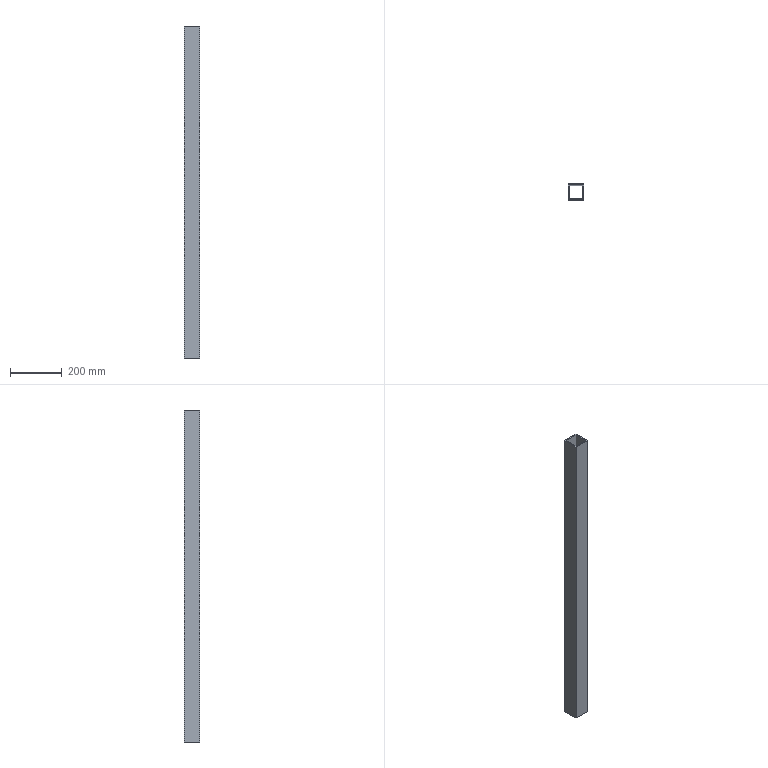Part | STEP file | ASND-0110-E63-HLTP01气SpringLower机架.3 | 1 solid | 10 faces | box 60 x 60 x 1280 mm | volume 1146880 mm3 | plane 10
STEP:
#1=CARTESIAN_POINT('',(0.,0.,0.));
#2=DIRECTION('',(0.,0.,1.));
#3=DIRECTION('',(1.,0.,0.));
#4=AXIS2_PLACEMENT_3D('',#1,#2,#3);
#5=CARTESIAN_POINT('',(-710.,-525.,1280.));
#6=VERTEX_POINT('',#5);
#7=CARTESIAN_POINT('',(-710.,-465.,1280.));
#8=VERTEX_POINT('',#7);
#9=CARTESIAN_POINT('',(-710.,-525.,1280.));
#10=DIRECTION('',(0.,1.,0.));
#11=VECTOR('',#10,1.);
#12=LINE('',#9,#11);
#13=CARTESIAN_POINT('',(-710.,-525.,1364.853));
#14=DIRECTION('',(-1.,0.,0.));
#15=DIRECTION('',(0.,0.7071,0.7071));
#16=AXIS2_PLACEMENT_3D('',#13,#14,#15);
#17=PLANE('',#16);
#18=CARTESIAN_POINT('',(-60.,60.));
#19=DIRECTION('',(0.7071,0.7071));
#20=VECTOR('',#19,1.);
#21=LINE('',#18,#20);
#22=(GEOMETRIC_REPRESENTATION_CONTEXT(2)PARAMETRIC_REPRESENTATION_CONTEXT()REPRESENTATION_CONTEXT('',''));
#23=DEFINITIONAL_REPRESENTATION('',(#21),#22);
#24=PCURVE('',#17,#23);
#25=CARTESIAN_POINT('',(-1564.853,-465.,1280.));
#26=DIRECTION('',(0.,0.,1.));
#27=DIRECTION('',(0.7071,0.7071,0.));
#28=AXIS2_PLACEMENT_3D('',#25,#26,#27);
#29=PLANE('',#28);
#30=CARTESIAN_POINT('',(562.046,-646.899));
#31=DIRECTION('',(0.7071,0.7071));
#32=VECTOR('',#31,1.);
#33=LINE('',#30,#32);
#34=(GEOMETRIC_REPRESENTATION_CONTEXT(2)PARAMETRIC_REPRESENTATION_CONTEXT()REPRESENTATION_CONTEXT('',''));
#35=DEFINITIONAL_REPRESENTATION('',(#33),#34);
#36=PCURVE('',#29,#35);
#37=SURFACE_CURVE('',#12,(#24,#36),.PCURVE_S1.);
#38=EDGE_CURVE('',#6,#8,#37,.T.);
#39=ORIENTED_EDGE('',*,*,#38,.F.);
#40=CARTESIAN_POINT('',(-710.,-525.,0.));
#41=VERTEX_POINT('',#40);
#42=CARTESIAN_POINT('',(-710.,-525.,1280.));
#43=DIRECTION('',(0.,0.,-1.));
#44=VECTOR('',#43,1.);
#45=LINE('',#42,#44);
#46=CARTESIAN_POINT('',(-60.,60.));
#47=DIRECTION('',(-0.7071,0.7071));
#48=VECTOR('',#47,1.);
#49=LINE('',#46,#48);
#50=(GEOMETRIC_REPRESENTATION_CONTEXT(2)PARAMETRIC_REPRESENTATION_CONTEXT()REPRESENTATION_CONTEXT('',''));
#51=DEFINITIONAL_REPRESENTATION('',(#49),#50);
#52=PCURVE('',#17,#51);
#53=CARTESIAN_POINT('',(-770.,-525.,1364.853));
#54=DIRECTION('',(0.,1.,0.));
#55=DIRECTION('',(0.7071,0.,0.7071));
#56=AXIS2_PLACEMENT_3D('',#53,#54,#55);
#57=PLANE('',#56);
#58=CARTESIAN_POINT('',(-17.574,102.426));
#59=DIRECTION('',(-0.7071,0.7071));
#60=VECTOR('',#59,1.);
#61=LINE('',#58,#60);
#62=(GEOMETRIC_REPRESENTATION_CONTEXT(2)PARAMETRIC_REPRESENTATION_CONTEXT()REPRESENTATION_CONTEXT('',''));
#63=DEFINITIONAL_REPRESENTATION('',(#61),#62);
#64=PCURVE('',#57,#63);
#65=SURFACE_CURVE('',#45,(#52,#64),.PCURVE_S1.);
#66=EDGE_CURVE('',#6,#41,#65,.T.);
#67=ORIENTED_EDGE('',*,*,#66,.T.);
#68=CARTESIAN_POINT('',(-710.,-465.,0.));
#69=VERTEX_POINT('',#68);
#70=CARTESIAN_POINT('',(-710.,-525.,0.));
#71=DIRECTION('',(0.,1.,0.));
#72=VECTOR('',#71,1.);
#73=LINE('',#70,#72);
#74=CARTESIAN_POINT('',(-965.097,965.097));
#75=DIRECTION('',(0.7071,0.7071));
#76=VECTOR('',#75,1.);
#77=LINE('',#74,#76);
#78=(GEOMETRIC_REPRESENTATION_CONTEXT(2)PARAMETRIC_REPRESENTATION_CONTEXT()REPRESENTATION_CONTEXT('',''));
#79=DEFINITIONAL_REPRESENTATION('',(#77),#78);
#80=PCURVE('',#17,#79);
#81=CARTESIAN_POINT('',(0.,0.,0.));
#82=DIRECTION('',(0.,0.,1.));
#83=DIRECTION('',(0.7071,0.7071,0.));
#84=AXIS2_PLACEMENT_3D('',#81,#82,#83);
#85=PLANE('',#84);
#86=CARTESIAN_POINT('',(-873.277,130.815));
#87=DIRECTION('',(0.7071,0.7071));
#88=VECTOR('',#87,1.);
#89=LINE('',#86,#88);
#90=(GEOMETRIC_REPRESENTATION_CONTEXT(2)PARAMETRIC_REPRESENTATION_CONTEXT()REPRESENTATION_CONTEXT('',''));
#91=DEFINITIONAL_REPRESENTATION('',(#89),#90);
#92=PCURVE('',#85,#91);
#93=SURFACE_CURVE('',#73,(#80,#92),.PCURVE_S1.);
#94=EDGE_CURVE('',#41,#69,#93,.T.);
#95=ORIENTED_EDGE('',*,*,#94,.T.);
#96=CARTESIAN_POINT('',(-710.,-465.,1280.));
#97=DIRECTION('',(0.,0.,-1.));
#98=VECTOR('',#97,1.);
#99=LINE('',#96,#98);
#100=CARTESIAN_POINT('',(-17.574,102.426));
#101=DIRECTION('',(-0.7071,0.7071));
#102=VECTOR('',#101,1.);
#103=LINE('',#100,#102);
#104=(GEOMETRIC_REPRESENTATION_CONTEXT(2)PARAMETRIC_REPRESENTATION_CONTEXT()REPRESENTATION_CONTEXT('',''));
#105=DEFINITIONAL_REPRESENTATION('',(#103),#104);
#106=PCURVE('',#17,#105);
#107=CARTESIAN_POINT('',(-710.,-465.,1364.853));
#108=DIRECTION('',(0.,-1.,0.));
#109=DIRECTION('',(0.7071,0.,0.7071));
#110=AXIS2_PLACEMENT_3D('',#107,#108,#109);
#111=PLANE('',#110);
#112=CARTESIAN_POINT('',(-60.,-60.));
#113=DIRECTION('',(-0.7071,-0.7071));
#114=VECTOR('',#113,1.);
#115=LINE('',#112,#114);
#116=(GEOMETRIC_REPRESENTATION_CONTEXT(2)PARAMETRIC_REPRESENTATION_CONTEXT()REPRESENTATION_CONTEXT('',''));
#117=DEFINITIONAL_REPRESENTATION('',(#115),#116);
#118=PCURVE('',#111,#117);
#119=SURFACE_CURVE('',#99,(#106,#118),.PCURVE_S1.);
#120=EDGE_CURVE('',#8,#69,#119,.T.);
#121=ORIENTED_EDGE('',*,*,#120,.F.);
#122=EDGE_LOOP('',(#39,#67,#95,#121));
#123=FACE_BOUND('',#122,.T.);
#124=ADVANCED_FACE('',(#123),#17,.F.);
#125=CARTESIAN_POINT('',(-770.,-525.,1280.));
#126=VERTEX_POINT('',#125);
#127=CARTESIAN_POINT('',(-770.,-525.,1280.));
#128=DIRECTION('',(1.,0.,0.));
#129=VECTOR('',#128,1.);
#130=LINE('',#127,#129);
#131=CARTESIAN_POINT('',(-60.,60.));
#132=DIRECTION('',(0.7071,0.7071));
#133=VECTOR('',#132,1.);
#134=LINE('',#131,#133);
#135=(GEOMETRIC_REPRESENTATION_CONTEXT(2)PARAMETRIC_REPRESENTATION_CONTEXT()REPRESENTATION_CONTEXT('',''));
#136=DEFINITIONAL_REPRESENTATION('',(#134),#135);
#137=PCURVE('',#57,#136);
#138=CARTESIAN_POINT('',(519.619,-604.472));
#139=DIRECTION('',(0.7071,-0.7071));
#140=VECTOR('',#139,1.);
#141=LINE('',#138,#140);
#142=(GEOMETRIC_REPRESENTATION_CONTEXT(2)PARAMETRIC_REPRESENTATION_CONTEXT()REPRESENTATION_CONTEXT('',''));
#143=DEFINITIONAL_REPRESENTATION('',(#141),#142);
#144=PCURVE('',#29,#143);
#145=SURFACE_CURVE('',#130,(#137,#144),.PCURVE_S1.);
#146=EDGE_CURVE('',#126,#6,#145,.T.);
#147=ORIENTED_EDGE('',*,*,#146,.F.);
#148=CARTESIAN_POINT('',(-770.,-525.,0.));
#149=VERTEX_POINT('',#148);
#150=CARTESIAN_POINT('',(-770.,-525.,1280.));
#151=DIRECTION('',(0.,0.,-1.));
#152=VECTOR('',#151,1.);
#153=LINE('',#150,#152);
#154=CARTESIAN_POINT('',(-60.,60.));
#155=DIRECTION('',(-0.7071,0.7071));
#156=VECTOR('',#155,1.);
#157=LINE('',#154,#156);
#158=(GEOMETRIC_REPRESENTATION_CONTEXT(2)PARAMETRIC_REPRESENTATION_CONTEXT()REPRESENTATION_CONTEXT('',''));
#159=DEFINITIONAL_REPRESENTATION('',(#157),#158);
#160=PCURVE('',#57,#159);
#161=CARTESIAN_POINT('',(-770.,-465.,1364.853));
#162=DIRECTION('',(1.,0.,0.));
#163=DIRECTION('',(0.,0.7071,0.7071));
#164=AXIS2_PLACEMENT_3D('',#161,#162,#163);
#165=PLANE('',#164);
#166=CARTESIAN_POINT('',(-102.426,-17.574));
#167=DIRECTION('',(-0.7071,-0.7071));
#168=VECTOR('',#167,1.);
#169=LINE('',#166,#168);
#170=(GEOMETRIC_REPRESENTATION_CONTEXT(2)PARAMETRIC_REPRESENTATION_CONTEXT()REPRESENTATION_CONTEXT('',''));
#171=DEFINITIONAL_REPRESENTATION('',(#169),#170);
#172=PCURVE('',#165,#171);
#173=SURFACE_CURVE('',#153,(#160,#172),.PCURVE_S1.);
#174=EDGE_CURVE('',#126,#149,#173,.T.);
#175=ORIENTED_EDGE('',*,*,#174,.T.);
#176=CARTESIAN_POINT('',(-770.,-525.,0.));
#177=DIRECTION('',(1.,0.,0.));
#178=VECTOR('',#177,1.);
#179=LINE('',#176,#178);
#180=CARTESIAN_POINT('',(-965.097,965.097));
#181=DIRECTION('',(0.7071,0.7071));
#182=VECTOR('',#181,1.);
#183=LINE('',#180,#182);
#184=(GEOMETRIC_REPRESENTATION_CONTEXT(2)PARAMETRIC_REPRESENTATION_CONTEXT()REPRESENTATION_CONTEXT('',''));
#185=DEFINITIONAL_REPRESENTATION('',(#183),#184);
#186=PCURVE('',#57,#185);
#187=CARTESIAN_POINT('',(-915.703,173.241));
#188=DIRECTION('',(0.7071,-0.7071));
#189=VECTOR('',#188,1.);
#190=LINE('',#187,#189);
#191=(GEOMETRIC_REPRESENTATION_CONTEXT(2)PARAMETRIC_REPRESENTATION_CONTEXT()REPRESENTATION_CONTEXT('',''));
#192=DEFINITIONAL_REPRESENTATION('',(#190),#191);
#193=PCURVE('',#85,#192);
#194=SURFACE_CURVE('',#179,(#186,#193),.PCURVE_S1.);
#195=EDGE_CURVE('',#149,#41,#194,.T.);
#196=ORIENTED_EDGE('',*,*,#195,.T.);
#197=ORIENTED_EDGE('',*,*,#66,.F.);
#198=EDGE_LOOP('',(#147,#175,#196,#197));
#199=FACE_BOUND('',#198,.T.);
#200=ADVANCED_FACE('',(#199),#57,.F.);
#201=CARTESIAN_POINT('',(-770.,-465.,1280.));
#202=VERTEX_POINT('',#201);
#203=CARTESIAN_POINT('',(-770.,-465.,1280.));
#204=DIRECTION('',(0.,-1.,0.));
#205=VECTOR('',#204,1.);
#206=LINE('',#203,#205);
#207=CARTESIAN_POINT('',(-60.,-60.));
#208=DIRECTION('',(-0.7071,0.7071));
#209=VECTOR('',#208,1.);
#210=LINE('',#207,#209);
#211=(GEOMETRIC_REPRESENTATION_CONTEXT(2)PARAMETRIC_REPRESENTATION_CONTEXT()REPRESENTATION_CONTEXT('',''));
#212=DEFINITIONAL_REPRESENTATION('',(#210),#211);
#213=PCURVE('',#165,#212);
#214=CARTESIAN_POINT('',(562.046,-562.046));
#215=DIRECTION('',(-0.7071,-0.7071));
#216=VECTOR('',#215,1.);
#217=LINE('',#214,#216);
#218=(GEOMETRIC_REPRESENTATION_CONTEXT(2)PARAMETRIC_REPRESENTATION_CONTEXT()REPRESENTATION_CONTEXT('',''));
#219=DEFINITIONAL_REPRESENTATION('',(#217),#218);
#220=PCURVE('',#29,#219);
#221=SURFACE_CURVE('',#206,(#213,#220),.PCURVE_S1.);
#222=EDGE_CURVE('',#202,#126,#221,.T.);
#223=ORIENTED_EDGE('',*,*,#222,.F.);
#224=CARTESIAN_POINT('',(-770.,-465.,0.));
#225=VERTEX_POINT('',#224);
#226=CARTESIAN_POINT('',(-770.,-465.,1280.));
#227=DIRECTION('',(0.,0.,-1.));
#228=VECTOR('',#227,1.);
#229=LINE('',#226,#228);
#230=CARTESIAN_POINT('',(-60.,-60.));
#231=DIRECTION('',(-0.7071,-0.7071));
#232=VECTOR('',#231,1.);
#233=LINE('',#230,#232);
#234=(GEOMETRIC_REPRESENTATION_CONTEXT(2)PARAMETRIC_REPRESENTATION_CONTEXT()REPRESENTATION_CONTEXT('',''));
#235=DEFINITIONAL_REPRESENTATION('',(#233),#234);
#236=PCURVE('',#165,#235);
#237=CARTESIAN_POINT('',(-102.426,-17.574));
#238=DIRECTION('',(-0.7071,-0.7071));
#239=VECTOR('',#238,1.);
#240=LINE('',#237,#239);
#241=(GEOMETRIC_REPRESENTATION_CONTEXT(2)PARAMETRIC_REPRESENTATION_CONTEXT()REPRESENTATION_CONTEXT('',''));
#242=DEFINITIONAL_REPRESENTATION('',(#240),#241);
#243=PCURVE('',#111,#242);
#244=SURFACE_CURVE('',#229,(#236,#243),.PCURVE_S1.);
#245=EDGE_CURVE('',#202,#225,#244,.T.);
#246=ORIENTED_EDGE('',*,*,#245,.T.);
#247=CARTESIAN_POINT('',(-770.,-465.,0.));
#248=DIRECTION('',(0.,-1.,0.));
#249=VECTOR('',#248,1.);
#250=LINE('',#247,#249);
#251=CARTESIAN_POINT('',(-965.097,-965.097));
#252=DIRECTION('',(-0.7071,0.7071));
#253=VECTOR('',#252,1.);
#254=LINE('',#251,#253);
#255=(GEOMETRIC_REPRESENTATION_CONTEXT(2)PARAMETRIC_REPRESENTATION_CONTEXT()REPRESENTATION_CONTEXT('',''));
#256=DEFINITIONAL_REPRESENTATION('',(#254),#255);
#257=PCURVE('',#165,#256);
#258=CARTESIAN_POINT('',(-873.277,215.668));
#259=DIRECTION('',(-0.7071,-0.7071));
#260=VECTOR('',#259,1.);
#261=LINE('',#258,#260);
#262=(GEOMETRIC_REPRESENTATION_CONTEXT(2)PARAMETRIC_REPRESENTATION_CONTEXT()REPRESENTATION_CONTEXT('',''));
#263=DEFINITIONAL_REPRESENTATION('',(#261),#262);
#264=PCURVE('',#85,#263);
#265=SURFACE_CURVE('',#250,(#257,#264),.PCURVE_S1.);
#266=EDGE_CURVE('',#225,#149,#265,.T.);
#267=ORIENTED_EDGE('',*,*,#266,.T.);
#268=ORIENTED_EDGE('',*,*,#174,.F.);
#269=EDGE_LOOP('',(#223,#246,#267,#268));
#270=FACE_BOUND('',#269,.T.);
#271=ADVANCED_FACE('',(#270),#165,.F.);
#272=CARTESIAN_POINT('',(-710.,-465.,1280.));
#273=DIRECTION('',(-1.,0.,0.));
#274=VECTOR('',#273,1.);
#275=LINE('',#272,#274);
#276=CARTESIAN_POINT('',(-60.,-60.));
#277=DIRECTION('',(-0.7071,0.7071));
#278=VECTOR('',#277,1.);
#279=LINE('',#276,#278);
#280=(GEOMETRIC_REPRESENTATION_CONTEXT(2)PARAMETRIC_REPRESENTATION_CONTEXT()REPRESENTATION_CONTEXT('',''));
#281=DEFINITIONAL_REPRESENTATION('',(#279),#280);
#282=PCURVE('',#111,#281);
#283=CARTESIAN_POINT('',(604.472,-604.472));
#284=DIRECTION('',(-0.7071,0.7071));
#285=VECTOR('',#284,1.);
#286=LINE('',#283,#285);
#287=(GEOMETRIC_REPRESENTATION_CONTEXT(2)PARAMETRIC_REPRESENTATION_CONTEXT()REPRESENTATION_CONTEXT('',''));
#288=DEFINITIONAL_REPRESENTATION('',(#286),#287);
#289=PCURVE('',#29,#288);
#290=SURFACE_CURVE('',#275,(#282,#289),.PCURVE_S1.);
#291=EDGE_CURVE('',#8,#202,#290,.T.);
#292=ORIENTED_EDGE('',*,*,#291,.F.);
#293=ORIENTED_EDGE('',*,*,#120,.T.);
#294=CARTESIAN_POINT('',(-710.,-465.,0.));
#295=DIRECTION('',(-1.,0.,0.));
#296=VECTOR('',#295,1.);
#297=LINE('',#294,#296);
#298=CARTESIAN_POINT('',(-965.097,-965.097));
#299=DIRECTION('',(-0.7071,0.7071));
#300=VECTOR('',#299,1.);
#301=LINE('',#298,#300);
#302=(GEOMETRIC_REPRESENTATION_CONTEXT(2)PARAMETRIC_REPRESENTATION_CONTEXT()REPRESENTATION_CONTEXT('',''));
#303=DEFINITIONAL_REPRESENTATION('',(#301),#302);
#304=PCURVE('',#111,#303);
#305=CARTESIAN_POINT('',(-830.85,173.241));
#306=DIRECTION('',(-0.7071,0.7071));
#307=VECTOR('',#306,1.);
#308=LINE('',#305,#307);
#309=(GEOMETRIC_REPRESENTATION_CONTEXT(2)PARAMETRIC_REPRESENTATION_CONTEXT()REPRESENTATION_CONTEXT('',''));
#310=DEFINITIONAL_REPRESENTATION('',(#308),#309);
#311=PCURVE('',#85,#310);
#312=SURFACE_CURVE('',#297,(#304,#311),.PCURVE_S1.);
#313=EDGE_CURVE('',#69,#225,#312,.T.);
#314=ORIENTED_EDGE('',*,*,#313,.T.);
#315=ORIENTED_EDGE('',*,*,#245,.F.);
#316=EDGE_LOOP('',(#292,#293,#314,#315));
#317=FACE_BOUND('',#316,.T.);
#318=ADVANCED_FACE('',(#317),#111,.F.);
#319=ORIENTED_EDGE('',*,*,#313,.F.);
#320=ORIENTED_EDGE('',*,*,#94,.F.);
#321=ORIENTED_EDGE('',*,*,#195,.F.);
#322=ORIENTED_EDGE('',*,*,#266,.F.);
#323=EDGE_LOOP('',(#319,#320,#321,#322));
#324=FACE_BOUND('',#323,.T.);
#325=CARTESIAN_POINT('',(-714.,-521.,0.));
#326=VERTEX_POINT('',#325);
#327=CARTESIAN_POINT('',(-714.,-469.,0.));
#328=VERTEX_POINT('',#327);
#329=CARTESIAN_POINT('',(-714.,-521.,0.));
#330=DIRECTION('',(0.,1.,0.));
#331=VECTOR('',#330,1.);
#332=LINE('',#329,#331);
#333=CARTESIAN_POINT('',(-873.277,136.472));
#334=DIRECTION('',(0.7071,0.7071));
#335=VECTOR('',#334,1.);
#336=LINE('',#333,#335);
#337=(GEOMETRIC_REPRESENTATION_CONTEXT(2)PARAMETRIC_REPRESENTATION_CONTEXT()REPRESENTATION_CONTEXT('',''));
#338=DEFINITIONAL_REPRESENTATION('',(#336),#337);
#339=PCURVE('',#85,#338);
#340=CARTESIAN_POINT('',(-714.,-521.,1364.853));
#341=DIRECTION('',(-1.,0.,0.));
#342=DIRECTION('',(0.,0.7071,0.7071));
#343=AXIS2_PLACEMENT_3D('',#340,#341,#342);
#344=PLANE('',#343);
#345=CARTESIAN_POINT('',(-965.097,965.097));
#346=DIRECTION('',(0.7071,0.7071));
#347=VECTOR('',#346,1.);
#348=LINE('',#345,#347);
#349=(GEOMETRIC_REPRESENTATION_CONTEXT(2)PARAMETRIC_REPRESENTATION_CONTEXT()REPRESENTATION_CONTEXT('',''));
#350=DEFINITIONAL_REPRESENTATION('',(#348),#349);
#351=PCURVE('',#344,#350);
#352=SURFACE_CURVE('',#332,(#339,#351),.PCURVE_S1.);
#353=EDGE_CURVE('',#326,#328,#352,.T.);
#354=ORIENTED_EDGE('',*,*,#353,.T.);
#355=CARTESIAN_POINT('',(-766.,-469.,0.));
#356=VERTEX_POINT('',#355);
#357=CARTESIAN_POINT('',(-714.,-469.,0.));
#358=DIRECTION('',(-1.,0.,0.));
#359=VECTOR('',#358,1.);
#360=LINE('',#357,#359);
#361=CARTESIAN_POINT('',(-836.507,173.241));
#362=DIRECTION('',(-0.7071,0.7071));
#363=VECTOR('',#362,1.);
#364=LINE('',#361,#363);
#365=(GEOMETRIC_REPRESENTATION_CONTEXT(2)PARAMETRIC_REPRESENTATION_CONTEXT()REPRESENTATION_CONTEXT('',''));
#366=DEFINITIONAL_REPRESENTATION('',(#364),#365);
#367=PCURVE('',#85,#366);
#368=CARTESIAN_POINT('',(-714.,-469.,1364.853));
#369=DIRECTION('',(0.,-1.,0.));
#370=DIRECTION('',(0.7071,0.,0.7071));
#371=AXIS2_PLACEMENT_3D('',#368,#369,#370);
#372=PLANE('',#371);
#373=CARTESIAN_POINT('',(-965.097,-965.097));
#374=DIRECTION('',(-0.7071,0.7071));
#375=VECTOR('',#374,1.);
#376=LINE('',#373,#375);
#377=(GEOMETRIC_REPRESENTATION_CONTEXT(2)PARAMETRIC_REPRESENTATION_CONTEXT()REPRESENTATION_CONTEXT('',''));
#378=DEFINITIONAL_REPRESENTATION('',(#376),#377);
#379=PCURVE('',#372,#378);
#380=SURFACE_CURVE('',#360,(#367,#379),.PCURVE_S1.);
#381=EDGE_CURVE('',#328,#356,#380,.T.);
#382=ORIENTED_EDGE('',*,*,#381,.T.);
#383=CARTESIAN_POINT('',(-766.,-521.,0.));
#384=VERTEX_POINT('',#383);
#385=CARTESIAN_POINT('',(-766.,-469.,0.));
#386=DIRECTION('',(0.,-1.,0.));
#387=VECTOR('',#386,1.);
#388=LINE('',#385,#387);
#389=CARTESIAN_POINT('',(-873.277,210.011));
#390=DIRECTION('',(-0.7071,-0.7071));
#391=VECTOR('',#390,1.);
#392=LINE('',#389,#391);
#393=(GEOMETRIC_REPRESENTATION_CONTEXT(2)PARAMETRIC_REPRESENTATION_CONTEXT()REPRESENTATION_CONTEXT('',''));
#394=DEFINITIONAL_REPRESENTATION('',(#392),#393);
#395=PCURVE('',#85,#394);
#396=CARTESIAN_POINT('',(-766.,-469.,1364.853));
#397=DIRECTION('',(1.,0.,0.));
#398=DIRECTION('',(0.,0.7071,0.7071));
#399=AXIS2_PLACEMENT_3D('',#396,#397,#398);
#400=PLANE('',#399);
#401=CARTESIAN_POINT('',(-965.097,-965.097));
#402=DIRECTION('',(-0.7071,0.7071));
#403=VECTOR('',#402,1.);
#404=LINE('',#401,#403);
#405=(GEOMETRIC_REPRESENTATION_CONTEXT(2)PARAMETRIC_REPRESENTATION_CONTEXT()REPRESENTATION_CONTEXT('',''));
#406=DEFINITIONAL_REPRESENTATION('',(#404),#405);
#407=PCURVE('',#400,#406);
#408=SURFACE_CURVE('',#388,(#395,#407),.PCURVE_S1.);
#409=EDGE_CURVE('',#356,#384,#408,.T.);
#410=ORIENTED_EDGE('',*,*,#409,.T.);
#411=CARTESIAN_POINT('',(-766.,-521.,0.));
#412=DIRECTION('',(1.,0.,0.));
#413=VECTOR('',#412,1.);
#414=LINE('',#411,#413);
#415=CARTESIAN_POINT('',(-910.046,173.241));
#416=DIRECTION('',(0.7071,-0.7071));
#417=VECTOR('',#416,1.);
#418=LINE('',#415,#417);
#419=(GEOMETRIC_REPRESENTATION_CONTEXT(2)PARAMETRIC_REPRESENTATION_CONTEXT()REPRESENTATION_CONTEXT('',''));
#420=DEFINITIONAL_REPRESENTATION('',(#418),#419);
#421=PCURVE('',#85,#420);
#422=CARTESIAN_POINT('',(-766.,-521.,1364.853));
#423=DIRECTION('',(0.,1.,0.));
#424=DIRECTION('',(0.7071,0.,0.7071));
#425=AXIS2_PLACEMENT_3D('',#422,#423,#424);
#426=PLANE('',#425);
#427=CARTESIAN_POINT('',(-965.097,965.097));
#428=DIRECTION('',(0.7071,0.7071));
#429=VECTOR('',#428,1.);
#430=LINE('',#427,#429);
#431=(GEOMETRIC_REPRESENTATION_CONTEXT(2)PARAMETRIC_REPRESENTATION_CONTEXT()REPRESENTATION_CONTEXT('',''));
#432=DEFINITIONAL_REPRESENTATION('',(#430),#431);
#433=PCURVE('',#426,#432);
#434=SURFACE_CURVE('',#414,(#421,#433),.PCURVE_S1.);
#435=EDGE_CURVE('',#384,#326,#434,.T.);
#436=ORIENTED_EDGE('',*,*,#435,.T.);
#437=EDGE_LOOP('',(#354,#382,#410,#436));
#438=FACE_BOUND('',#437,.T.);
#439=ADVANCED_FACE('',(#324,#438),#85,.F.);
#440=CARTESIAN_POINT('',(-766.,-521.,1280.));
#441=VERTEX_POINT('',#440);
#442=CARTESIAN_POINT('',(-766.,-521.,1280.));
#443=DIRECTION('',(0.,0.,-1.));
#444=VECTOR('',#443,1.);
#445=LINE('',#442,#444);
#446=CARTESIAN_POINT('',(-60.,60.));
#447=DIRECTION('',(-0.7071,0.7071));
#448=VECTOR('',#447,1.);
#449=LINE('',#446,#448);
#450=(GEOMETRIC_REPRESENTATION_CONTEXT(2)PARAMETRIC_REPRESENTATION_CONTEXT()REPRESENTATION_CONTEXT('',''));
#451=DEFINITIONAL_REPRESENTATION('',(#449),#450);
#452=PCURVE('',#426,#451);
#453=CARTESIAN_POINT('',(-96.77,-23.23));
#454=DIRECTION('',(-0.7071,-0.7071));
#455=VECTOR('',#454,1.);
#456=LINE('',#453,#455);
#457=(GEOMETRIC_REPRESENTATION_CONTEXT(2)PARAMETRIC_REPRESENTATION_CONTEXT()REPRESENTATION_CONTEXT('',''));
#458=DEFINITIONAL_REPRESENTATION('',(#456),#457);
#459=PCURVE('',#400,#458);
#460=SURFACE_CURVE('',#445,(#452,#459),.PCURVE_S1.);
#461=EDGE_CURVE('',#441,#384,#460,.T.);
#462=ORIENTED_EDGE('',*,*,#461,.F.);
#463=CARTESIAN_POINT('',(-714.,-521.,1280.));
#464=VERTEX_POINT('',#463);
#465=CARTESIAN_POINT('',(-766.,-521.,1280.));
#466=DIRECTION('',(1.,0.,0.));
#467=VECTOR('',#466,1.);
#468=LINE('',#465,#467);
#469=CARTESIAN_POINT('',(-60.,60.));
#470=DIRECTION('',(0.7071,0.7071));
#471=VECTOR('',#470,1.);
#472=LINE('',#469,#471);
#473=(GEOMETRIC_REPRESENTATION_CONTEXT(2)PARAMETRIC_REPRESENTATION_CONTEXT()REPRESENTATION_CONTEXT('',''));
#474=DEFINITIONAL_REPRESENTATION('',(#472),#473);
#475=PCURVE('',#426,#474);
#476=CARTESIAN_POINT('',(525.276,-604.472));
#477=DIRECTION('',(0.7071,-0.7071));
#478=VECTOR('',#477,1.);
#479=LINE('',#476,#478);
#480=(GEOMETRIC_REPRESENTATION_CONTEXT(2)PARAMETRIC_REPRESENTATION_CONTEXT()REPRESENTATION_CONTEXT('',''));
#481=DEFINITIONAL_REPRESENTATION('',(#479),#480);
#482=PCURVE('',#29,#481);
#483=SURFACE_CURVE('',#468,(#475,#482),.PCURVE_S1.);
#484=EDGE_CURVE('',#441,#464,#483,.T.);
#485=ORIENTED_EDGE('',*,*,#484,.T.);
#486=CARTESIAN_POINT('',(-714.,-521.,1280.));
#487=DIRECTION('',(0.,0.,-1.));
#488=VECTOR('',#487,1.);
#489=LINE('',#486,#488);
#490=CARTESIAN_POINT('',(-23.23,96.77));
#491=DIRECTION('',(-0.7071,0.7071));
#492=VECTOR('',#491,1.);
#493=LINE('',#490,#492);
#494=(GEOMETRIC_REPRESENTATION_CONTEXT(2)PARAMETRIC_REPRESENTATION_CONTEXT()REPRESENTATION_CONTEXT('',''));
#495=DEFINITIONAL_REPRESENTATION('',(#493),#494);
#496=PCURVE('',#426,#495);
#497=CARTESIAN_POINT('',(-60.,60.));
#498=DIRECTION('',(-0.7071,0.7071));
#499=VECTOR('',#498,1.);
#500=LINE('',#497,#499);
#501=(GEOMETRIC_REPRESENTATION_CONTEXT(2)PARAMETRIC_REPRESENTATION_CONTEXT()REPRESENTATION_CONTEXT('',''));
#502=DEFINITIONAL_REPRESENTATION('',(#500),#501);
#503=PCURVE('',#344,#502);
#504=SURFACE_CURVE('',#489,(#496,#503),.PCURVE_S1.);
#505=EDGE_CURVE('',#464,#326,#504,.T.);
#506=ORIENTED_EDGE('',*,*,#505,.T.);
#507=ORIENTED_EDGE('',*,*,#435,.F.);
#508=EDGE_LOOP('',(#462,#485,#506,#507));
#509=FACE_BOUND('',#508,.T.);
#510=ADVANCED_FACE('',(#509),#426,.T.);
#511=CARTESIAN_POINT('',(-766.,-469.,1280.));
#512=VERTEX_POINT('',#511);
#513=CARTESIAN_POINT('',(-766.,-469.,1280.));
#514=DIRECTION('',(0.,0.,-1.));
#515=VECTOR('',#514,1.);
#516=LINE('',#513,#515);
#517=CARTESIAN_POINT('',(-60.,-60.));
#518=DIRECTION('',(-0.7071,-0.7071));
#519=VECTOR('',#518,1.);
#520=LINE('',#517,#519);
#521=(GEOMETRIC_REPRESENTATION_CONTEXT(2)PARAMETRIC_REPRESENTATION_CONTEXT()REPRESENTATION_CONTEXT('',''));
#522=DEFINITIONAL_REPRESENTATION('',(#520),#521);
#523=PCURVE('',#400,#522);
#524=CARTESIAN_POINT('',(-96.77,-23.23));
#525=DIRECTION('',(-0.7071,-0.7071));
#526=VECTOR('',#525,1.);
#527=LINE('',#524,#526);
#528=(GEOMETRIC_REPRESENTATION_CONTEXT(2)PARAMETRIC_REPRESENTATION_CONTEXT()REPRESENTATION_CONTEXT('',''));
#529=DEFINITIONAL_REPRESENTATION('',(#527),#528);
#530=PCURVE('',#372,#529);
#531=SURFACE_CURVE('',#516,(#523,#530),.PCURVE_S1.);
#532=EDGE_CURVE('',#512,#356,#531,.T.);
#533=ORIENTED_EDGE('',*,*,#532,.F.);
#534=CARTESIAN_POINT('',(-766.,-469.,1280.));
#535=DIRECTION('',(0.,-1.,0.));
#536=VECTOR('',#535,1.);
#537=LINE('',#534,#536);
#538=CARTESIAN_POINT('',(-60.,-60.));
#539=DIRECTION('',(-0.7071,0.7071));
#540=VECTOR('',#539,1.);
#541=LINE('',#538,#540);
#542=(GEOMETRIC_REPRESENTATION_CONTEXT(2)PARAMETRIC_REPRESENTATION_CONTEXT()REPRESENTATION_CONTEXT('',''));
#543=DEFINITIONAL_REPRESENTATION('',(#541),#542);
#544=PCURVE('',#400,#543);
#545=CARTESIAN_POINT('',(562.046,-567.703));
#546=DIRECTION('',(-0.7071,-0.7071));
#547=VECTOR('',#546,1.);
#548=LINE('',#545,#547);
#549=(GEOMETRIC_REPRESENTATION_CONTEXT(2)PARAMETRIC_REPRESENTATION_CONTEXT()REPRESENTATION_CONTEXT('',''));
#550=DEFINITIONAL_REPRESENTATION('',(#548),#549);
#551=PCURVE('',#29,#550);
#552=SURFACE_CURVE('',#537,(#544,#551),.PCURVE_S1.);
#553=EDGE_CURVE('',#512,#441,#552,.T.);
#554=ORIENTED_EDGE('',*,*,#553,.T.);
#555=ORIENTED_EDGE('',*,*,#461,.T.);
#556=ORIENTED_EDGE('',*,*,#409,.F.);
#557=EDGE_LOOP('',(#533,#554,#555,#556));
#558=FACE_BOUND('',#557,.T.);
#559=ADVANCED_FACE('',(#558),#400,.T.);
#560=CARTESIAN_POINT('',(-714.,-469.,1280.));
#561=VERTEX_POINT('',#560);
#562=CARTESIAN_POINT('',(-714.,-469.,1280.));
#563=DIRECTION('',(0.,0.,-1.));
#564=VECTOR('',#563,1.);
#565=LINE('',#562,#564);
#566=CARTESIAN_POINT('',(-60.,-60.));
#567=DIRECTION('',(-0.7071,-0.7071));
#568=VECTOR('',#567,1.);
#569=LINE('',#566,#568);
#570=(GEOMETRIC_REPRESENTATION_CONTEXT(2)PARAMETRIC_REPRESENTATION_CONTEXT()REPRESENTATION_CONTEXT('',''));
#571=DEFINITIONAL_REPRESENTATION('',(#569),#570);
#572=PCURVE('',#372,#571);
#573=CARTESIAN_POINT('',(-23.23,96.77));
#574=DIRECTION('',(-0.7071,0.7071));
#575=VECTOR('',#574,1.);
#576=LINE('',#573,#575);
#577=(GEOMETRIC_REPRESENTATION_CONTEXT(2)PARAMETRIC_REPRESENTATION_CONTEXT()REPRESENTATION_CONTEXT('',''));
#578=DEFINITIONAL_REPRESENTATION('',(#576),#577);
#579=PCURVE('',#344,#578);
#580=SURFACE_CURVE('',#565,(#572,#579),.PCURVE_S1.);
#581=EDGE_CURVE('',#561,#328,#580,.T.);
#582=ORIENTED_EDGE('',*,*,#581,.F.);
#583=CARTESIAN_POINT('',(-714.,-469.,1280.));
#584=DIRECTION('',(-1.,0.,0.));
#585=VECTOR('',#584,1.);
#586=LINE('',#583,#585);
#587=CARTESIAN_POINT('',(-60.,-60.));
#588=DIRECTION('',(-0.7071,0.7071));
#589=VECTOR('',#588,1.);
#590=LINE('',#587,#589);
#591=(GEOMETRIC_REPRESENTATION_CONTEXT(2)PARAMETRIC_REPRESENTATION_CONTEXT()REPRESENTATION_CONTEXT('',''));
#592=DEFINITIONAL_REPRESENTATION('',(#590),#591);
#593=PCURVE('',#372,#592);
#594=CARTESIAN_POINT('',(598.815,-604.472));
#595=DIRECTION('',(-0.7071,0.7071));
#596=VECTOR('',#595,1.);
#597=LINE('',#594,#596);
#598=(GEOMETRIC_REPRESENTATION_CONTEXT(2)PARAMETRIC_REPRESENTATION_CONTEXT()REPRESENTATION_CONTEXT('',''));
#599=DEFINITIONAL_REPRESENTATION('',(#597),#598);
#600=PCURVE('',#29,#599);
#601=SURFACE_CURVE('',#586,(#593,#600),.PCURVE_S1.);
#602=EDGE_CURVE('',#561,#512,#601,.T.);
#603=ORIENTED_EDGE('',*,*,#602,.T.);
#604=ORIENTED_EDGE('',*,*,#532,.T.);
#605=ORIENTED_EDGE('',*,*,#381,.F.);
#606=EDGE_LOOP('',(#582,#603,#604,#605));
#607=FACE_BOUND('',#606,.T.);
#608=ADVANCED_FACE('',(#607),#372,.T.);
#609=ORIENTED_EDGE('',*,*,#505,.F.);
#610=CARTESIAN_POINT('',(-714.,-521.,1280.));
#611=DIRECTION('',(0.,1.,0.));
#612=VECTOR('',#611,1.);
#613=LINE('',#610,#612);
#614=CARTESIAN_POINT('',(-60.,60.));
#615=DIRECTION('',(0.7071,0.7071));
#616=VECTOR('',#615,1.);
#617=LINE('',#614,#616);
#618=(GEOMETRIC_REPRESENTATION_CONTEXT(2)PARAMETRIC_REPRESENTATION_CONTEXT()REPRESENTATION_CONTEXT('',''));
#619=DEFINITIONAL_REPRESENTATION('',(#617),#618);
#620=PCURVE('',#344,#619);
#621=CARTESIAN_POINT('',(562.046,-641.242));
#622=DIRECTION('',(0.7071,0.7071));
#623=VECTOR('',#622,1.);
#624=LINE('',#621,#623);
#625=(GEOMETRIC_REPRESENTATION_CONTEXT(2)PARAMETRIC_REPRESENTATION_CONTEXT()REPRESENTATION_CONTEXT('',''));
#626=DEFINITIONAL_REPRESENTATION('',(#624),#625);
#627=PCURVE('',#29,#626);
#628=SURFACE_CURVE('',#613,(#620,#627),.PCURVE_S1.);
#629=EDGE_CURVE('',#464,#561,#628,.T.);
#630=ORIENTED_EDGE('',*,*,#629,.T.);
#631=ORIENTED_EDGE('',*,*,#581,.T.);
#632=ORIENTED_EDGE('',*,*,#353,.F.);
#633=EDGE_LOOP('',(#609,#630,#631,#632));
#634=FACE_BOUND('',#633,.T.);
#635=ADVANCED_FACE('',(#634),#344,.T.);
#636=ORIENTED_EDGE('',*,*,#222,.T.);
#637=ORIENTED_EDGE('',*,*,#146,.T.);
#638=ORIENTED_EDGE('',*,*,#38,.T.);
#639=ORIENTED_EDGE('',*,*,#291,.T.);
#640=EDGE_LOOP('',(#636,#637,#638,#639));
#641=FACE_BOUND('',#640,.T.);
#642=ORIENTED_EDGE('',*,*,#484,.F.);
#643=ORIENTED_EDGE('',*,*,#553,.F.);
#644=ORIENTED_EDGE('',*,*,#602,.F.);
#645=ORIENTED_EDGE('',*,*,#629,.F.);
#646=EDGE_LOOP('',(#642,#643,#644,#645));
#647=FACE_BOUND('',#646,.T.);
#648=ADVANCED_FACE('',(#641,#647),#29,.T.);
#649=CLOSED_SHELL('',(#124,#200,#271,#318,#439,#510,#559,#608,#635,#648));
#650=MANIFOLD_SOLID_BREP('',#649);
#651=(LENGTH_UNIT()NAMED_UNIT(*)SI_UNIT(.MILLI.,.METRE.));
#652=UNCERTAINTY_MEASURE_WITH_UNIT(LENGTH_MEASURE(0.0000001),#651,'','');
#653=(NAMED_UNIT(*)PLANE_ANGLE_UNIT()SI_UNIT($,.RADIAN.));
#654=(NAMED_UNIT(*)SI_UNIT($,.STERADIAN.)SOLID_ANGLE_UNIT());
#655=(GEOMETRIC_REPRESENTATION_CONTEXT(3)GLOBAL_UNCERTAINTY_ASSIGNED_CONTEXT((#652))GLOBAL_UNIT_ASSIGNED_CONTEXT((#651,#653,#654))REPRESENTATION_CONTEXT('',''));
#656=ADVANCED_BREP_SHAPE_REPRESENTATION('',(#4,#650),#655);